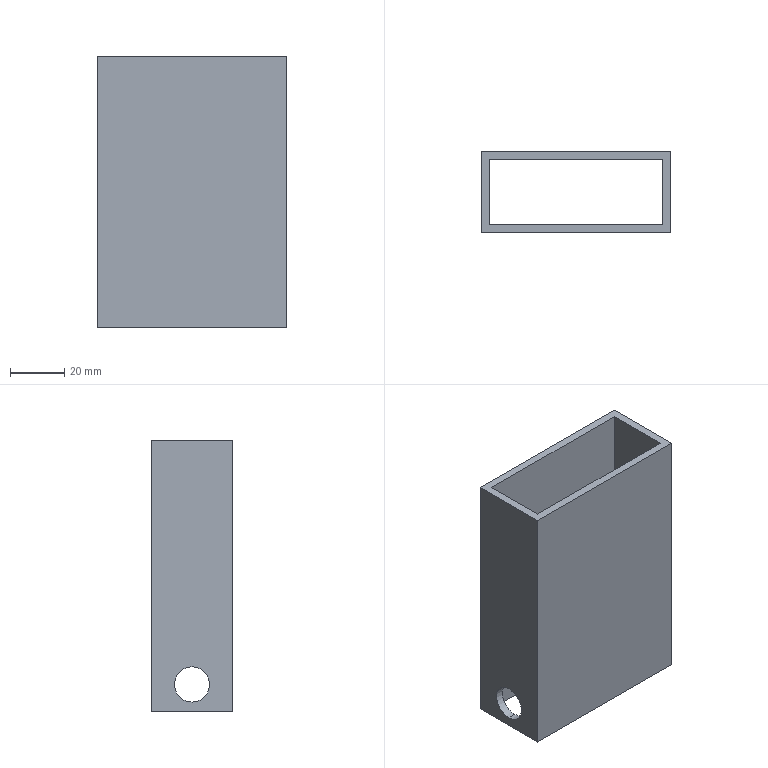Part | SolidWorks | features Extrusion 1, ICE 1, Shell 1 | 1 solid | 14 faces | box 70 x 30 x 100 mm | volume 55604 mm3 | plane 10 | cylinder 4 | commonest cylinder face diameters 13 x4
STEP:
#1=CARTESIAN_POINT('',(70.,15.,3.5));
#2=VERTEX_POINT('',#1);
#3=CARTESIAN_POINT('',(70.,15.,16.5));
#4=VERTEX_POINT('',#3);
#5=CARTESIAN_POINT('',(70.,15.,10.));
#6=DIRECTION('',(-1.,0.,0.));
#7=DIRECTION('',(0.,0.,1.));
#8=AXIS2_PLACEMENT_3D('',#5,#6,#7);
#9=CIRCLE('',#8,6.5);
#10=EDGE_CURVE('',#2,#4,#9,.T.);
#11=ORIENTED_EDGE('',*,*,#10,.F.);
#12=CARTESIAN_POINT('',(67.,15.,3.5));
#13=VERTEX_POINT('',#12);
#14=CARTESIAN_POINT('',(100.,15.,3.5));
#15=DIRECTION('',(-1.,0.,0.));
#16=VECTOR('',#15,1000.);
#17=LINE('',#14,#16);
#18=EDGE_CURVE('',#2,#13,#17,.T.);
#19=ORIENTED_EDGE('',*,*,#18,.T.);
#20=CARTESIAN_POINT('',(67.,15.,16.5));
#21=VERTEX_POINT('',#20);
#22=CARTESIAN_POINT('',(67.,15.,10.));
#23=DIRECTION('',(-1.,0.,0.));
#24=DIRECTION('',(0.,0.,1.));
#25=AXIS2_PLACEMENT_3D('',#22,#23,#24);
#26=CIRCLE('',#25,6.5);
#27=EDGE_CURVE('',#13,#21,#26,.T.);
#28=ORIENTED_EDGE('',*,*,#27,.T.);
#29=CARTESIAN_POINT('',(100.,15.,16.5));
#30=DIRECTION('',(-1.,0.,0.));
#31=VECTOR('',#30,1000.);
#32=LINE('',#29,#31);
#33=EDGE_CURVE('',#4,#21,#32,.T.);
#34=ORIENTED_EDGE('',*,*,#33,.F.);
#35=EDGE_LOOP('',(#11,#19,#28,#34));
#36=FACE_OUTER_BOUND('',#35,.T.);
#37=CARTESIAN_POINT('',(100.,15.,10.));
#38=DIRECTION('',(-1.,0.,0.));
#39=DIRECTION('',(0.,0.,1.));
#40=AXIS2_PLACEMENT_3D('',#37,#38,#39);
#41=CYLINDRICAL_SURFACE('',#40,6.5);
#42=ADVANCED_FACE('',(#36),#41,.F.);
#43=CARTESIAN_POINT('',(3.,15.,16.5));
#44=VERTEX_POINT('',#43);
#45=CARTESIAN_POINT('',(3.,15.,3.5));
#46=VERTEX_POINT('',#45);
#47=CARTESIAN_POINT('',(3.,15.,10.));
#48=DIRECTION('',(1.,0.,0.));
#49=DIRECTION('',(0.,0.,-1.));
#50=AXIS2_PLACEMENT_3D('',#47,#48,#49);
#51=CIRCLE('',#50,6.5);
#52=EDGE_CURVE('',#44,#46,#51,.T.);
#53=ORIENTED_EDGE('',*,*,#52,.T.);
#54=CARTESIAN_POINT('',(0.,15.,3.5));
#55=VERTEX_POINT('',#54);
#56=CARTESIAN_POINT('',(100.,15.,3.5));
#57=DIRECTION('',(-1.,0.,0.));
#58=VECTOR('',#57,1000.);
#59=LINE('',#56,#58);
#60=EDGE_CURVE('',#46,#55,#59,.T.);
#61=ORIENTED_EDGE('',*,*,#60,.T.);
#62=CARTESIAN_POINT('',(0.,15.,16.5));
#63=VERTEX_POINT('',#62);
#64=CARTESIAN_POINT('',(0.,15.,10.));
#65=DIRECTION('',(-1.,0.,0.));
#66=DIRECTION('',(0.,0.,1.));
#67=AXIS2_PLACEMENT_3D('',#64,#65,#66);
#68=CIRCLE('',#67,6.5);
#69=EDGE_CURVE('',#55,#63,#68,.T.);
#70=ORIENTED_EDGE('',*,*,#69,.T.);
#71=CARTESIAN_POINT('',(100.,15.,16.5));
#72=DIRECTION('',(-1.,0.,0.));
#73=VECTOR('',#72,1000.);
#74=LINE('',#71,#73);
#75=EDGE_CURVE('',#44,#63,#74,.T.);
#76=ORIENTED_EDGE('',*,*,#75,.F.);
#77=EDGE_LOOP('',(#53,#61,#70,#76));
#78=FACE_OUTER_BOUND('',#77,.T.);
#79=CARTESIAN_POINT('',(100.,15.,10.));
#80=DIRECTION('',(-1.,0.,0.));
#81=DIRECTION('',(0.,0.,1.));
#82=AXIS2_PLACEMENT_3D('',#79,#80,#81);
#83=CYLINDRICAL_SURFACE('',#82,6.5);
#84=ADVANCED_FACE('',(#78),#83,.F.);
#85=CARTESIAN_POINT('',(0.,0.,100.));
#86=VERTEX_POINT('',#85);
#87=CARTESIAN_POINT('',(70.,0.,100.));
#88=VERTEX_POINT('',#87);
#89=CARTESIAN_POINT('',(70.,0.,100.));
#90=DIRECTION('',(1.,0.,0.));
#91=VECTOR('',#90,1000.);
#92=LINE('',#89,#91);
#93=EDGE_CURVE('',#86,#88,#92,.T.);
#94=ORIENTED_EDGE('',*,*,#93,.T.);
#95=CARTESIAN_POINT('',(70.,30.,100.));
#96=VERTEX_POINT('',#95);
#97=CARTESIAN_POINT('',(70.,30.,100.));
#98=DIRECTION('',(0.,1.,0.));
#99=VECTOR('',#98,1000.);
#100=LINE('',#97,#99);
#101=EDGE_CURVE('',#88,#96,#100,.T.);
#102=ORIENTED_EDGE('',*,*,#101,.T.);
#103=CARTESIAN_POINT('',(0.,30.,100.));
#104=VERTEX_POINT('',#103);
#105=CARTESIAN_POINT('',(0.,30.,100.));
#106=DIRECTION('',(-1.,0.,0.));
#107=VECTOR('',#106,1000.);
#108=LINE('',#105,#107);
#109=EDGE_CURVE('',#96,#104,#108,.T.);
#110=ORIENTED_EDGE('',*,*,#109,.T.);
#111=CARTESIAN_POINT('',(0.,0.,100.));
#112=DIRECTION('',(0.,-1.,0.));
#113=VECTOR('',#112,1000.);
#114=LINE('',#111,#113);
#115=EDGE_CURVE('',#104,#86,#114,.T.);
#116=ORIENTED_EDGE('',*,*,#115,.T.);
#117=EDGE_LOOP('',(#94,#102,#110,#116));
#118=FACE_OUTER_BOUND('',#117,.T.);
#119=CARTESIAN_POINT('',(3.,3.,100.));
#120=VERTEX_POINT('',#119);
#121=CARTESIAN_POINT('',(67.,3.,100.));
#122=VERTEX_POINT('',#121);
#123=CARTESIAN_POINT('',(0.,3.,100.));
#124=DIRECTION('',(1.,0.,0.));
#125=VECTOR('',#124,1000.);
#126=LINE('',#123,#125);
#127=EDGE_CURVE('',#120,#122,#126,.T.);
#128=ORIENTED_EDGE('',*,*,#127,.F.);
#129=CARTESIAN_POINT('',(3.,27.,100.));
#130=VERTEX_POINT('',#129);
#131=CARTESIAN_POINT('',(3.,0.,100.));
#132=DIRECTION('',(0.,-1.,0.));
#133=VECTOR('',#132,1000.);
#134=LINE('',#131,#133);
#135=EDGE_CURVE('',#130,#120,#134,.T.);
#136=ORIENTED_EDGE('',*,*,#135,.F.);
#137=CARTESIAN_POINT('',(67.,27.,100.));
#138=VERTEX_POINT('',#137);
#139=CARTESIAN_POINT('',(0.,27.,100.));
#140=DIRECTION('',(-1.,0.,0.));
#141=VECTOR('',#140,1000.);
#142=LINE('',#139,#141);
#143=EDGE_CURVE('',#138,#130,#142,.T.);
#144=ORIENTED_EDGE('',*,*,#143,.F.);
#145=CARTESIAN_POINT('',(67.,0.,100.));
#146=DIRECTION('',(0.,1.,0.));
#147=VECTOR('',#146,1000.);
#148=LINE('',#145,#147);
#149=EDGE_CURVE('',#122,#138,#148,.T.);
#150=ORIENTED_EDGE('',*,*,#149,.F.);
#151=EDGE_LOOP('',(#128,#136,#144,#150));
#152=FACE_BOUND('',#151,.T.);
#153=CARTESIAN_POINT('',(0.,0.,100.));
#154=DIRECTION('',(0.,0.,-1.));
#155=DIRECTION('',(-1.,0.,0.));
#156=AXIS2_PLACEMENT_3D('',#153,#154,#155);
#157=PLANE('',#156);
#158=ADVANCED_FACE('',(#118,#152),#157,.F.);
#159=CARTESIAN_POINT('',(0.,0.,0.));
#160=VERTEX_POINT('',#159);
#161=CARTESIAN_POINT('',(70.,0.,0.));
#162=VERTEX_POINT('',#161);
#163=CARTESIAN_POINT('',(70.,0.,0.));
#164=DIRECTION('',(1.,0.,0.));
#165=VECTOR('',#164,1000.);
#166=LINE('',#163,#165);
#167=EDGE_CURVE('',#160,#162,#166,.T.);
#168=ORIENTED_EDGE('',*,*,#167,.F.);
#169=CARTESIAN_POINT('',(0.,30.,0.));
#170=VERTEX_POINT('',#169);
#171=CARTESIAN_POINT('',(0.,0.,0.));
#172=DIRECTION('',(0.,-1.,0.));
#173=VECTOR('',#172,1000.);
#174=LINE('',#171,#173);
#175=EDGE_CURVE('',#170,#160,#174,.T.);
#176=ORIENTED_EDGE('',*,*,#175,.F.);
#177=CARTESIAN_POINT('',(70.,30.,0.));
#178=VERTEX_POINT('',#177);
#179=CARTESIAN_POINT('',(0.,30.,0.));
#180=DIRECTION('',(-1.,0.,0.));
#181=VECTOR('',#180,1000.);
#182=LINE('',#179,#181);
#183=EDGE_CURVE('',#178,#170,#182,.T.);
#184=ORIENTED_EDGE('',*,*,#183,.F.);
#185=CARTESIAN_POINT('',(70.,30.,0.));
#186=DIRECTION('',(0.,1.,0.));
#187=VECTOR('',#186,1000.);
#188=LINE('',#185,#187);
#189=EDGE_CURVE('',#162,#178,#188,.T.);
#190=ORIENTED_EDGE('',*,*,#189,.F.);
#191=EDGE_LOOP('',(#168,#176,#184,#190));
#192=FACE_OUTER_BOUND('',#191,.T.);
#193=CARTESIAN_POINT('',(3.,27.,0.));
#194=VERTEX_POINT('',#193);
#195=CARTESIAN_POINT('',(3.,3.,0.));
#196=VERTEX_POINT('',#195);
#197=CARTESIAN_POINT('',(3.,0.,0.));
#198=DIRECTION('',(0.,-1.,0.));
#199=VECTOR('',#198,1000.);
#200=LINE('',#197,#199);
#201=EDGE_CURVE('',#194,#196,#200,.T.);
#202=ORIENTED_EDGE('',*,*,#201,.T.);
#203=CARTESIAN_POINT('',(67.,3.,0.));
#204=VERTEX_POINT('',#203);
#205=CARTESIAN_POINT('',(0.,3.,0.));
#206=DIRECTION('',(1.,0.,0.));
#207=VECTOR('',#206,1000.);
#208=LINE('',#205,#207);
#209=EDGE_CURVE('',#196,#204,#208,.T.);
#210=ORIENTED_EDGE('',*,*,#209,.T.);
#211=CARTESIAN_POINT('',(67.,27.,0.));
#212=VERTEX_POINT('',#211);
#213=CARTESIAN_POINT('',(67.,0.,0.));
#214=DIRECTION('',(0.,1.,0.));
#215=VECTOR('',#214,1000.);
#216=LINE('',#213,#215);
#217=EDGE_CURVE('',#204,#212,#216,.T.);
#218=ORIENTED_EDGE('',*,*,#217,.T.);
#219=CARTESIAN_POINT('',(0.,27.,0.));
#220=DIRECTION('',(-1.,0.,0.));
#221=VECTOR('',#220,1000.);
#222=LINE('',#219,#221);
#223=EDGE_CURVE('',#212,#194,#222,.T.);
#224=ORIENTED_EDGE('',*,*,#223,.T.);
#225=EDGE_LOOP('',(#202,#210,#218,#224));
#226=FACE_BOUND('',#225,.T.);
#227=CARTESIAN_POINT('',(0.,0.,0.));
#228=DIRECTION('',(0.,0.,-1.));
#229=DIRECTION('',(-1.,0.,0.));
#230=AXIS2_PLACEMENT_3D('',#227,#228,#229);
#231=PLANE('',#230);
#232=ADVANCED_FACE('',(#192,#226),#231,.T.);
#233=ORIENTED_EDGE('',*,*,#167,.T.);
#234=CARTESIAN_POINT('',(70.,0.,100.));
#235=DIRECTION('',(0.,0.,-1.));
#236=VECTOR('',#235,1000.);
#237=LINE('',#234,#236);
#238=EDGE_CURVE('',#88,#162,#237,.T.);
#239=ORIENTED_EDGE('',*,*,#238,.F.);
#240=ORIENTED_EDGE('',*,*,#93,.F.);
#241=CARTESIAN_POINT('',(0.,0.,100.));
#242=DIRECTION('',(0.,0.,-1.));
#243=VECTOR('',#242,1000.);
#244=LINE('',#241,#243);
#245=EDGE_CURVE('',#86,#160,#244,.T.);
#246=ORIENTED_EDGE('',*,*,#245,.T.);
#247=EDGE_LOOP('',(#233,#239,#240,#246));
#248=FACE_OUTER_BOUND('',#247,.T.);
#249=CARTESIAN_POINT('',(70.,0.,100.));
#250=DIRECTION('',(0.,1.,0.));
#251=DIRECTION('',(0.,0.,1.));
#252=AXIS2_PLACEMENT_3D('',#249,#250,#251);
#253=PLANE('',#252);
#254=ADVANCED_FACE('',(#248),#253,.F.);
#255=CARTESIAN_POINT('',(70.,15.,10.));
#256=DIRECTION('',(-1.,0.,0.));
#257=DIRECTION('',(0.,0.,1.));
#258=AXIS2_PLACEMENT_3D('',#255,#256,#257);
#259=CIRCLE('',#258,6.5);
#260=EDGE_CURVE('',#4,#2,#259,.T.);
#261=ORIENTED_EDGE('',*,*,#260,.T.);
#262=ORIENTED_EDGE('',*,*,#10,.T.);
#263=EDGE_LOOP('',(#261,#262));
#264=FACE_BOUND('',#263,.T.);
#265=ORIENTED_EDGE('',*,*,#189,.T.);
#266=CARTESIAN_POINT('',(70.,30.,100.));
#267=DIRECTION('',(0.,0.,-1.));
#268=VECTOR('',#267,1000.);
#269=LINE('',#266,#268);
#270=EDGE_CURVE('',#96,#178,#269,.T.);
#271=ORIENTED_EDGE('',*,*,#270,.F.);
#272=ORIENTED_EDGE('',*,*,#101,.F.);
#273=ORIENTED_EDGE('',*,*,#238,.T.);
#274=EDGE_LOOP('',(#265,#271,#272,#273));
#275=FACE_OUTER_BOUND('',#274,.T.);
#276=CARTESIAN_POINT('',(70.,30.,100.));
#277=DIRECTION('',(-1.,0.,0.));
#278=DIRECTION('',(0.,0.,1.));
#279=AXIS2_PLACEMENT_3D('',#276,#277,#278);
#280=PLANE('',#279);
#281=ADVANCED_FACE('',(#264,#275),#280,.F.);
#282=ORIENTED_EDGE('',*,*,#183,.T.);
#283=CARTESIAN_POINT('',(0.,30.,100.));
#284=DIRECTION('',(0.,0.,-1.));
#285=VECTOR('',#284,1000.);
#286=LINE('',#283,#285);
#287=EDGE_CURVE('',#104,#170,#286,.T.);
#288=ORIENTED_EDGE('',*,*,#287,.F.);
#289=ORIENTED_EDGE('',*,*,#109,.F.);
#290=ORIENTED_EDGE('',*,*,#270,.T.);
#291=EDGE_LOOP('',(#282,#288,#289,#290));
#292=FACE_OUTER_BOUND('',#291,.T.);
#293=CARTESIAN_POINT('',(0.,30.,100.));
#294=DIRECTION('',(0.,-1.,0.));
#295=DIRECTION('',(0.,0.,-1.));
#296=AXIS2_PLACEMENT_3D('',#293,#294,#295);
#297=PLANE('',#296);
#298=ADVANCED_FACE('',(#292),#297,.F.);
#299=CARTESIAN_POINT('',(0.,15.,10.));
#300=DIRECTION('',(-1.,0.,0.));
#301=DIRECTION('',(0.,0.,1.));
#302=AXIS2_PLACEMENT_3D('',#299,#300,#301);
#303=CIRCLE('',#302,6.5);
#304=EDGE_CURVE('',#63,#55,#303,.T.);
#305=ORIENTED_EDGE('',*,*,#304,.F.);
#306=ORIENTED_EDGE('',*,*,#69,.F.);
#307=EDGE_LOOP('',(#305,#306));
#308=FACE_BOUND('',#307,.T.);
#309=ORIENTED_EDGE('',*,*,#175,.T.);
#310=ORIENTED_EDGE('',*,*,#245,.F.);
#311=ORIENTED_EDGE('',*,*,#115,.F.);
#312=ORIENTED_EDGE('',*,*,#287,.T.);
#313=EDGE_LOOP('',(#309,#310,#311,#312));
#314=FACE_OUTER_BOUND('',#313,.T.);
#315=CARTESIAN_POINT('',(0.,0.,100.));
#316=DIRECTION('',(1.,0.,0.));
#317=DIRECTION('',(0.,0.,-1.));
#318=AXIS2_PLACEMENT_3D('',#315,#316,#317);
#319=PLANE('',#318);
#320=ADVANCED_FACE('',(#308,#314),#319,.F.);
#321=ORIENTED_EDGE('',*,*,#209,.F.);
#322=CARTESIAN_POINT('',(3.,3.,100.));
#323=DIRECTION('',(0.,0.,-1.));
#324=VECTOR('',#323,1000.);
#325=LINE('',#322,#324);
#326=EDGE_CURVE('',#120,#196,#325,.T.);
#327=ORIENTED_EDGE('',*,*,#326,.F.);
#328=ORIENTED_EDGE('',*,*,#127,.T.);
#329=CARTESIAN_POINT('',(67.,3.,100.));
#330=DIRECTION('',(0.,0.,-1.));
#331=VECTOR('',#330,1000.);
#332=LINE('',#329,#331);
#333=EDGE_CURVE('',#122,#204,#332,.T.);
#334=ORIENTED_EDGE('',*,*,#333,.T.);
#335=EDGE_LOOP('',(#321,#327,#328,#334));
#336=FACE_OUTER_BOUND('',#335,.T.);
#337=CARTESIAN_POINT('',(70.,3.,100.));
#338=DIRECTION('',(0.,1.,0.));
#339=DIRECTION('',(0.,0.,1.));
#340=AXIS2_PLACEMENT_3D('',#337,#338,#339);
#341=PLANE('',#340);
#342=ADVANCED_FACE('',(#336),#341,.T.);
#343=CARTESIAN_POINT('',(67.,15.,10.));
#344=DIRECTION('',(-1.,0.,0.));
#345=DIRECTION('',(0.,0.,1.));
#346=AXIS2_PLACEMENT_3D('',#343,#344,#345);
#347=CIRCLE('',#346,6.5);
#348=EDGE_CURVE('',#21,#13,#347,.T.);
#349=ORIENTED_EDGE('',*,*,#348,.F.);
#350=ORIENTED_EDGE('',*,*,#27,.F.);
#351=EDGE_LOOP('',(#349,#350));
#352=FACE_BOUND('',#351,.T.);
#353=ORIENTED_EDGE('',*,*,#217,.F.);
#354=ORIENTED_EDGE('',*,*,#333,.F.);
#355=ORIENTED_EDGE('',*,*,#149,.T.);
#356=CARTESIAN_POINT('',(67.,27.,100.));
#357=DIRECTION('',(0.,0.,-1.));
#358=VECTOR('',#357,1000.);
#359=LINE('',#356,#358);
#360=EDGE_CURVE('',#138,#212,#359,.T.);
#361=ORIENTED_EDGE('',*,*,#360,.T.);
#362=EDGE_LOOP('',(#353,#354,#355,#361));
#363=FACE_OUTER_BOUND('',#362,.T.);
#364=CARTESIAN_POINT('',(67.,30.,100.));
#365=DIRECTION('',(-1.,0.,0.));
#366=DIRECTION('',(0.,0.,1.));
#367=AXIS2_PLACEMENT_3D('',#364,#365,#366);
#368=PLANE('',#367);
#369=ADVANCED_FACE('',(#352,#363),#368,.T.);
#370=ORIENTED_EDGE('',*,*,#223,.F.);
#371=ORIENTED_EDGE('',*,*,#360,.F.);
#372=ORIENTED_EDGE('',*,*,#143,.T.);
#373=CARTESIAN_POINT('',(3.,27.,100.));
#374=DIRECTION('',(0.,0.,-1.));
#375=VECTOR('',#374,1000.);
#376=LINE('',#373,#375);
#377=EDGE_CURVE('',#130,#194,#376,.T.);
#378=ORIENTED_EDGE('',*,*,#377,.T.);
#379=EDGE_LOOP('',(#370,#371,#372,#378));
#380=FACE_OUTER_BOUND('',#379,.T.);
#381=CARTESIAN_POINT('',(0.,27.,100.));
#382=DIRECTION('',(0.,-1.,0.));
#383=DIRECTION('',(0.,0.,-1.));
#384=AXIS2_PLACEMENT_3D('',#381,#382,#383);
#385=PLANE('',#384);
#386=ADVANCED_FACE('',(#380),#385,.T.);
#387=ORIENTED_EDGE('',*,*,#52,.F.);
#388=CARTESIAN_POINT('',(3.,15.,10.));
#389=DIRECTION('',(1.,0.,0.));
#390=DIRECTION('',(0.,0.,-1.));
#391=AXIS2_PLACEMENT_3D('',#388,#389,#390);
#392=CIRCLE('',#391,6.5);
#393=EDGE_CURVE('',#46,#44,#392,.T.);
#394=ORIENTED_EDGE('',*,*,#393,.F.);
#395=EDGE_LOOP('',(#387,#394));
#396=FACE_BOUND('',#395,.T.);
#397=ORIENTED_EDGE('',*,*,#201,.F.);
#398=ORIENTED_EDGE('',*,*,#377,.F.);
#399=ORIENTED_EDGE('',*,*,#135,.T.);
#400=ORIENTED_EDGE('',*,*,#326,.T.);
#401=EDGE_LOOP('',(#397,#398,#399,#400));
#402=FACE_OUTER_BOUND('',#401,.T.);
#403=CARTESIAN_POINT('',(3.,0.,100.));
#404=DIRECTION('',(1.,0.,0.));
#405=DIRECTION('',(0.,0.,-1.));
#406=AXIS2_PLACEMENT_3D('',#403,#404,#405);
#407=PLANE('',#406);
#408=ADVANCED_FACE('',(#396,#402),#407,.T.);
#409=ORIENTED_EDGE('',*,*,#60,.F.);
#410=ORIENTED_EDGE('',*,*,#393,.T.);
#411=ORIENTED_EDGE('',*,*,#75,.T.);
#412=ORIENTED_EDGE('',*,*,#304,.T.);
#413=EDGE_LOOP('',(#409,#410,#411,#412));
#414=FACE_OUTER_BOUND('',#413,.T.);
#415=CARTESIAN_POINT('',(100.,15.,10.));
#416=DIRECTION('',(-1.,0.,0.));
#417=DIRECTION('',(0.,0.,1.));
#418=AXIS2_PLACEMENT_3D('',#415,#416,#417);
#419=CYLINDRICAL_SURFACE('',#418,6.5);
#420=ADVANCED_FACE('',(#414),#419,.F.);
#421=ORIENTED_EDGE('',*,*,#18,.F.);
#422=ORIENTED_EDGE('',*,*,#260,.F.);
#423=ORIENTED_EDGE('',*,*,#33,.T.);
#424=ORIENTED_EDGE('',*,*,#348,.T.);
#425=EDGE_LOOP('',(#421,#422,#423,#424));
#426=FACE_OUTER_BOUND('',#425,.T.);
#427=CARTESIAN_POINT('',(100.,15.,10.));
#428=DIRECTION('',(-1.,0.,0.));
#429=DIRECTION('',(0.,0.,1.));
#430=AXIS2_PLACEMENT_3D('',#427,#428,#429);
#431=CYLINDRICAL_SURFACE('',#430,6.5);
#432=ADVANCED_FACE('',(#426),#431,.F.);
#433=CLOSED_SHELL('',(#42,#84,#158,#232,#254,#281,#298,#320,#342,#369,#386,#408,#420,#432));
#434=MANIFOLD_SOLID_BREP('',#433);
#435=CARTESIAN_POINT('',(0.,0.,0.));
#436=DIRECTION('',(0.,0.,1.));
#437=DIRECTION('',(1.,0.,0.));
#438=AXIS2_PLACEMENT_3D('',#435,#436,#437);
#439=(LENGTH_UNIT()NAMED_UNIT(*)SI_UNIT(.MILLI.,.METRE.));
#440=UNCERTAINTY_MEASURE_WITH_UNIT(LENGTH_MEASURE(0.00001),#439,'','');
#441=(NAMED_UNIT(*)PLANE_ANGLE_UNIT()SI_UNIT($,.RADIAN.));
#442=(NAMED_UNIT(*)SI_UNIT($,.STERADIAN.)SOLID_ANGLE_UNIT());
#443=(GEOMETRIC_REPRESENTATION_CONTEXT(3)GLOBAL_UNCERTAINTY_ASSIGNED_CONTEXT((#440))GLOBAL_UNIT_ASSIGNED_CONTEXT((#439,#441,#442))REPRESENTATION_CONTEXT('',''));
#444=ADVANCED_BREP_SHAPE_REPRESENTATION('',(#434,#438),#443);